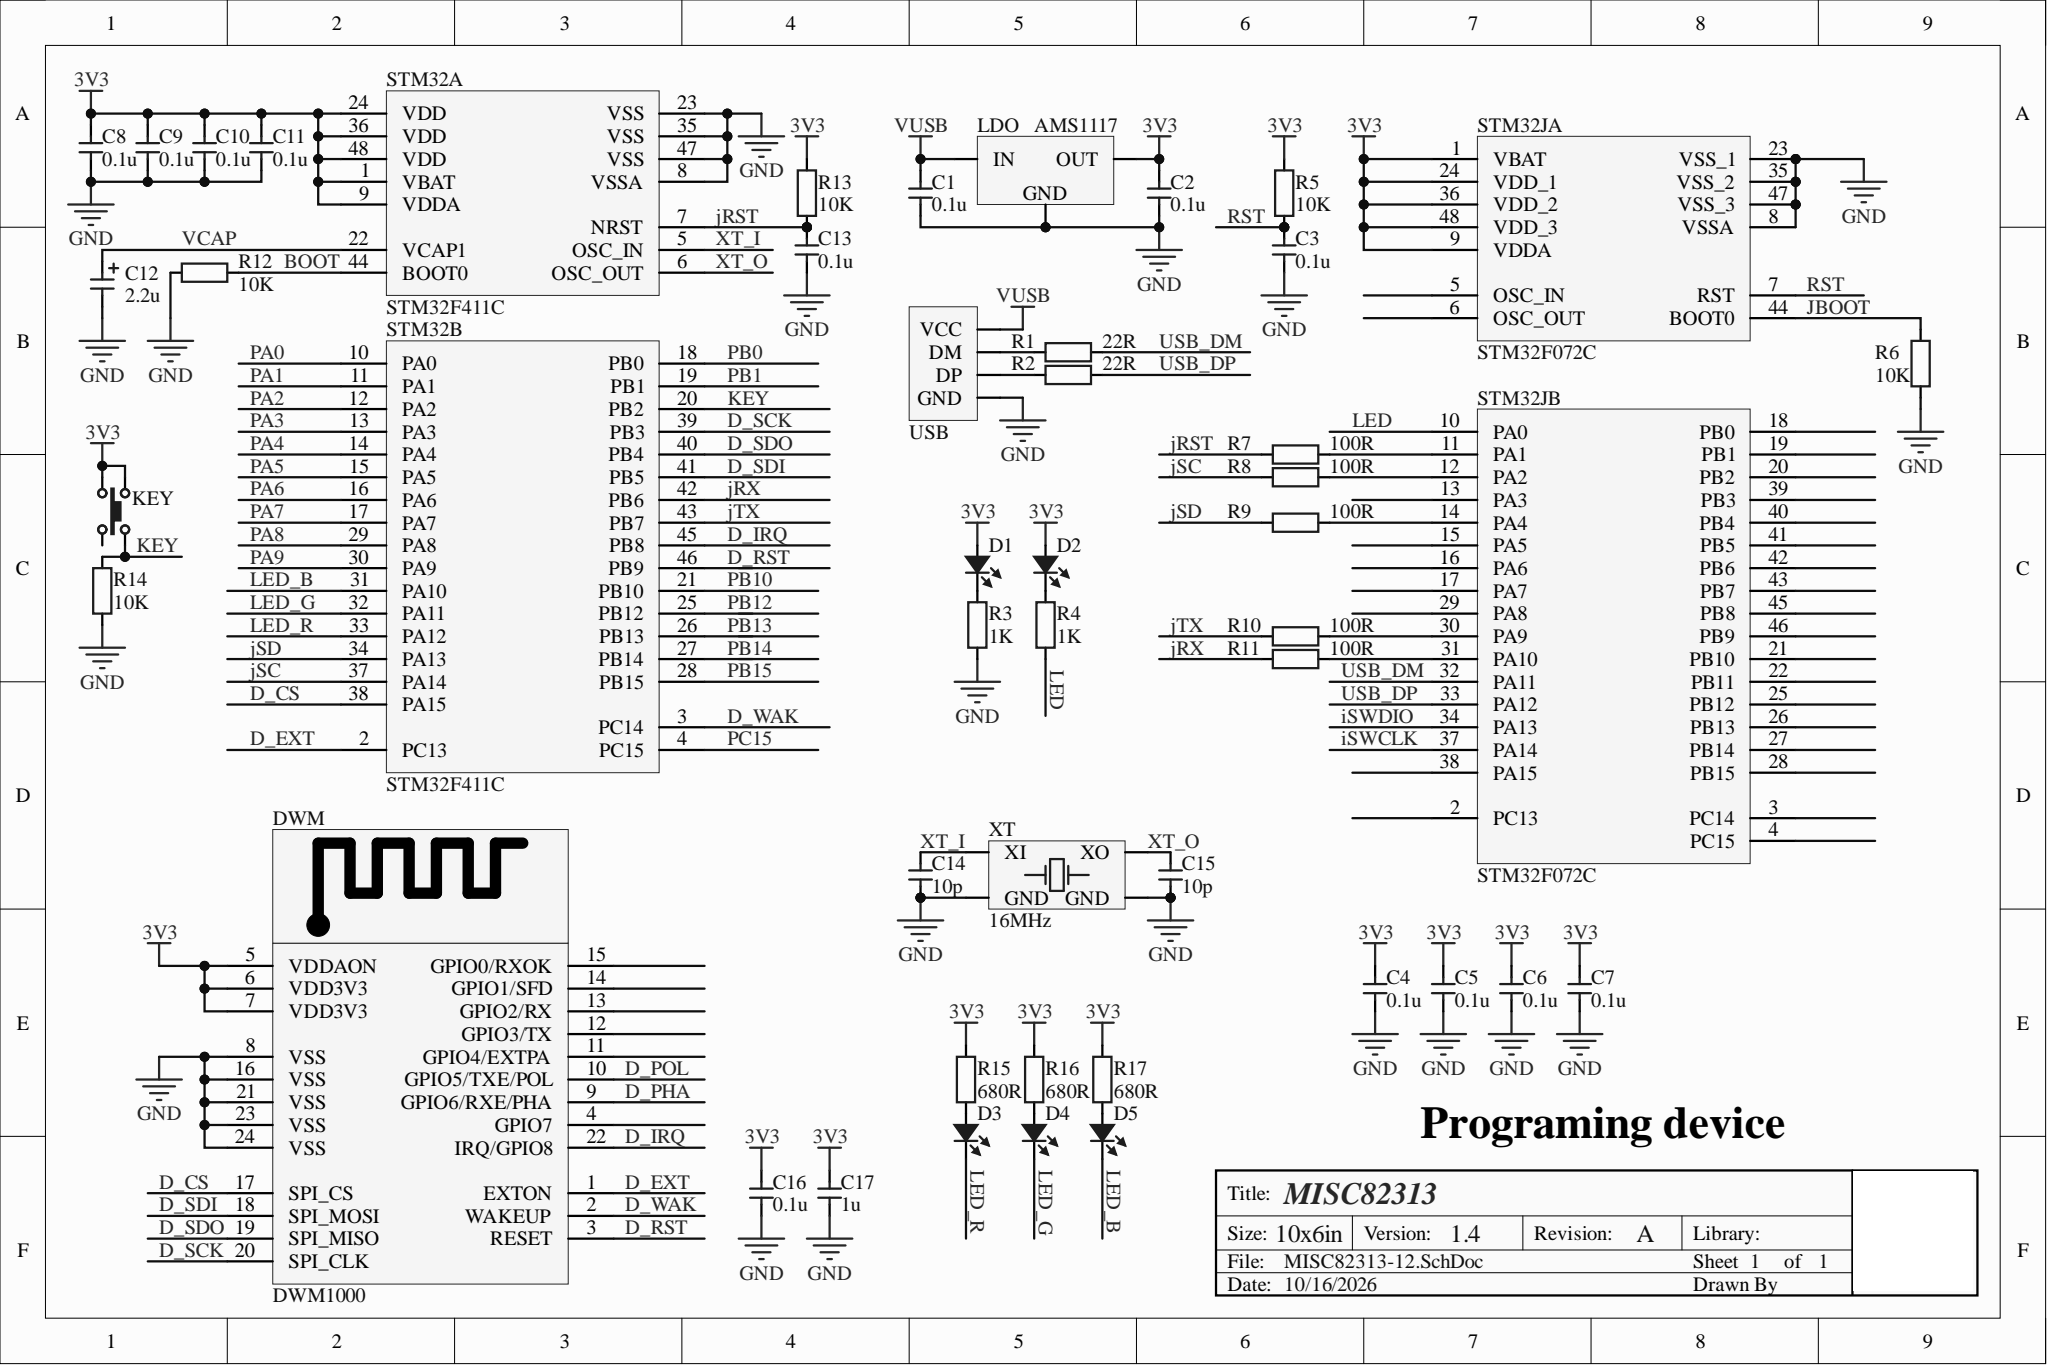Circuit board | Altium Designer | 46 parts | 41 nets
Bill of materials:
Comment,Description,Designator,Footprint,LibRef,Quantity
"Cap_0603","Capacitor","C1, C2, C3, C4, C5, C6, C7, C8, C9, C10, C11, C13, C14, C15, C16, C17","CAP_0603","Cap_0603","16"
"Cap_Tan_0805","Capacitor","C12","CAP_TAN_P0805","Cap_Tan_0805","1"
"LED_0603","LED","D1","LED_0603_YELLOW","LED_0603","1"
"LED_0603","LED","D2","LED_0603_ORANGE","LED_0603","1"
"LED_0603","LED","D3","LED_0603_RED","LED_0603","1"
"LED_0603","LED","D4","LED_0603_GREEN","LED_0603","1"
"LED_0603","LED","D5","LED_0603_BLUE","LED_0603","1"
"DWM1000","Module","DWM","DWM1000","DWM1000","1"
"ButtonTACT","Button","KEY","ButtonTACT_3.5*3.55_90","ButtonTACT","1"
"AMS1117","Power","LDO","SOT89-3","LDO1117","1"
"Res_0603","Resistor","R1, R2, R3, R4, R5, R6, R7, R8, R9, R10, R11, R12, R13, R14, R15, R16, R17","RES_0603","Res_0603","17"
"STM32F411C","MCU","STM32","QFN_P0.5_48","STM32F4x1C","1"
"STM32F072C","MCU","STM32J","LQFP_P0.5_48","STM32F103C","1"
"USB_Plug_TypeA","USB","USB","USB_Plug_TypeA","USB_Plug_TypeA","1"
"XTAL_2520_4P","Crystal Oscillator","XT","XT_2520_4","XTAL_2520_4P","1"
Netlist (Protel format):
[
C1
CAP_0603
Cap_0603



]
[
C2
CAP_0603
Cap_0603



]
[
C3
CAP_0603
Cap_0603



]
[
C4
CAP_0603
Cap_0603



]
[
C5
CAP_0603
Cap_0603



]
[
C6
CAP_0603
Cap_0603



]
[
C7
CAP_0603
Cap_0603



]
[
C8
CAP_0603
Cap_0603



]
[
C9
CAP_0603
Cap_0603



]
[
C10
CAP_0603
Cap_0603



]
[
C11
CAP_0603
Cap_0603



]
[
C12
CAP_TAN_P0805
Cap_Tan_0805



]
[
C13
CAP_0603
Cap_0603



]
[
C14
CAP_0603
Cap_0603



]
[
C15
CAP_0603
Cap_0603



]
[
C16
CAP_0603
Cap_0603



]
[
C17
CAP_0603
Cap_0603



]
[
D1
LED_0603_YELLOW
LED_0603



]
[
D2
LED_0603_ORANGE
LED_0603



]
[
D3
LED_0603_RED
LED_0603



]
[
D4
LED_0603_GREEN
LED_0603



]
[
D5
LED_0603_BLUE
LED_0603



]
[
DWM
DWM1000
DWM1000



]
[
KEY
ButtonTACT_3.5*3.55_90
ButtonTACT



]
[
LDO
SOT89-3
AMS1117



]
[
R1
RES_0603
Res_0603



]
[
R2
RES_0603
Res_0603



]
[
R3
RES_0603
Res_0603



]
[
R4
RES_0603
Res_0603



]
[
R5
RES_0603
Res_0603



]
[
R6
RES_0603
Res_0603



]
[
R7
RES_0603
Res_0603



]
[
R8
RES_0603
Res_0603



]
[
R9
RES_0603
Res_0603



]
[
R10
RES_0603
Res_0603



]
[
R11
RES_0603
Res_0603



]
[
R12
RES_0603
Res_0603



]
[
R13
RES_0603
Res_0603



]
[
R14
RES_0603
Res_0603



]
[
R15
RES_0603
Res_0603



]
[
R16
RES_0603
Res_0603



]
[
R17
RES_0603
Res_0603



]
[
STM32
QFN_P0.5_48
STM32F411C



]
[
STM32J
LQFP_P0.5_48
STM32F072C



]
[
USB
USB_Plug_TypeA
USB_Plug_TypeA



]
[
XT
XT_2520_4
XTAL_2520_4P



]
(
XT_O
C15-2
STM32-6
XT-3
)
(
XT_I
C14-2
STM32-5
XT-1
)
(
VUSB
C1-2
LDO-3
USB-1
)
(
VCAP
C12-1
STM32-22
)
(
USB_DP
R2-2
STM32J-33
)
(
USB_DM
R1-2
STM32J-32
)
(
RST
C3-2
R5-1
STM32J-7
)
(
NetR11_2
R11-2
STM32J-31
)
(
NetR10_2
R10-2
STM32J-30
)
(
NetR9_2
R9-2
STM32J-14
)
(
NetR8_2
R8-2
STM32J-12
)
(
NetR7_2
R7-2
STM32J-11
)
(
NetR2_1
R2-1
USB-3
)
(
NetR1_1
R1-1
USB-2
)
(
NetD5_1
D5-1
R17-1
)
(
NetD4_1
D4-1
R16-1
)
(
NetD3_1
D3-1
R15-1
)
(
NetD2_2
D2-2
R4-2
)
(
NetD1_2
D1-2
R3-2
)
(
LED_R
D3-2
STM32-33
)
(
LED_G
D4-2
STM32-32
)
(
LED_B
D5-2
STM32-31
)
(
LED
R4-1
STM32J-10
)
(
KEY
KEY-2
R14-2
STM32-20
)
(
jTX
R10-1
STM32-43
)
(
jSD
R9-1
STM32-34
)
(
jSC
R8-1
STM32-37
)
(
jRX
R11-1
STM32-42
)
(
jRST
C13-2
R7-1
R13-1
STM32-7
)
(
JBOOT
R6-2
STM32J-44
)
(
GND
C1-1
C2-1
C3-1
C4-1
C5-1
C6-1
C7-1
C8-1
C9-1
C10-1
C11-1
C12-2
C13-1
C14-1
C15-1
C16-2
C17-2
DWM-8
DWM-16
DWM-21
DWM-23
DWM-24
LDO-1
R3-1
R6-1
R12-2
R14-1
STM32-8
STM32-23
STM32-35
STM32-47
STM32J-8
STM32J-23
STM32J-35
STM32J-47
USB-4
XT-2
XT-4
)
(
D_WAK
DWM-2
STM32-3
)
(
D_SDO
DWM-19
STM32-40
)
(
D_SDI
DWM-18
STM32-41
)
(
D_SCK
DWM-20
STM32-39
)
(
D_RST
DWM-3
STM32-46
)
(
D_IRQ
DWM-22
STM32-45
)
(
D_EXT
DWM-1
STM32-2
)
(
D_CS
DWM-17
STM32-38
)
(
BOOT
R12-1
STM32-44
)
(
3V3
C2-2
C4-2
C5-2
C6-2
C7-2
C8-2
C9-2
C10-2
C11-2
C16-1
C17-1
D1-1
D2-1
DWM-5
DWM-6
DWM-7
KEY-1
KEY-3
LDO-2
R5-2
R13-2
R15-2
R16-2
R17-2
STM32-1
STM32-9
STM32-24
STM32-36
STM32-48
STM32J-1
STM32J-9
STM32J-24
STM32J-36
STM32J-48
)